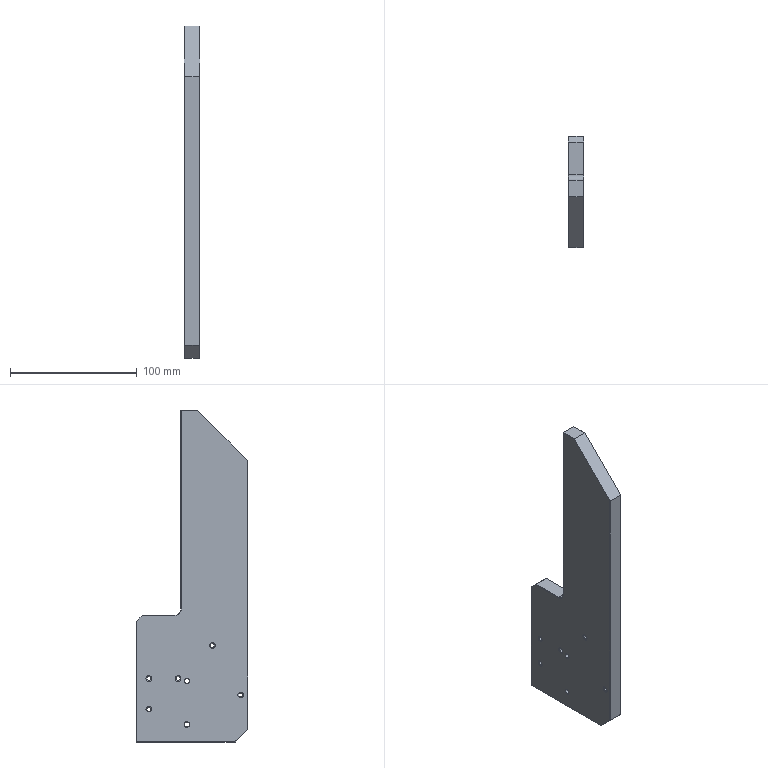Part | NX | 1 solid | 103 faces | box 12 x 88 x 262 mm | volume 196318 mm3 | cylinder 39 | cone 36 | plane 28 | commonest cylinder face diameters 3.3 x22 2.5 x8 4 x8 10 x1